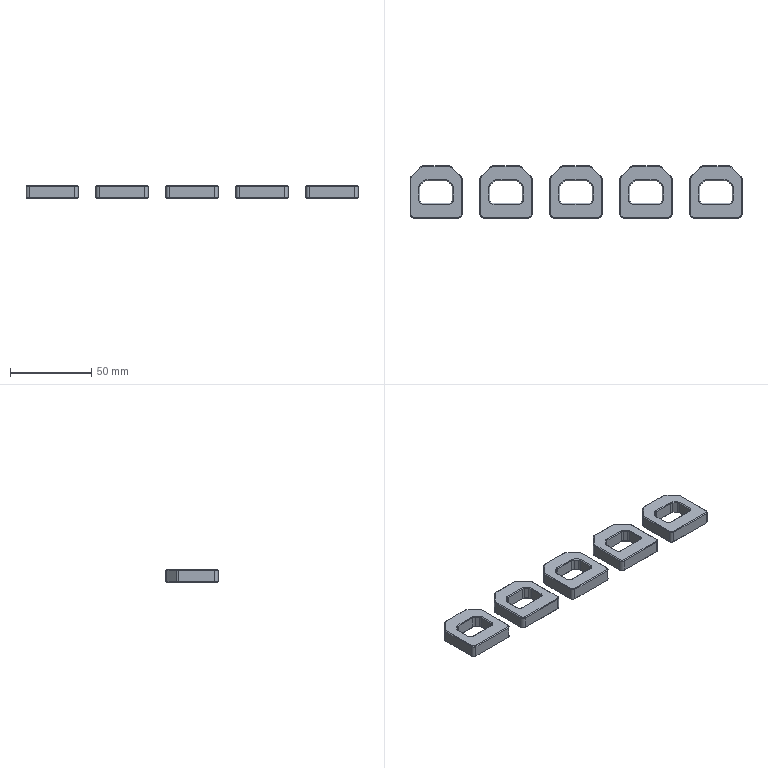NC program | NX | posted with a generic post | part box 204 x 32 x 8 mm
Lines 1 to 18 of 9506:
N10 G17 G21 G94 G90
(FLOOR_WALL , TOOL : D80)
N12 T19 M6
N14 G54
N16 G17 G0 G90 X-147. Y0. S6500 M3
N18 G43 Z30. H19
N20 Z3.
N22 G94 G1 Z0. F1500.
N24 X-144.
N26 X144.
N28 X147.
N30 Z3.
N32 G0 Z30.
N34 M5